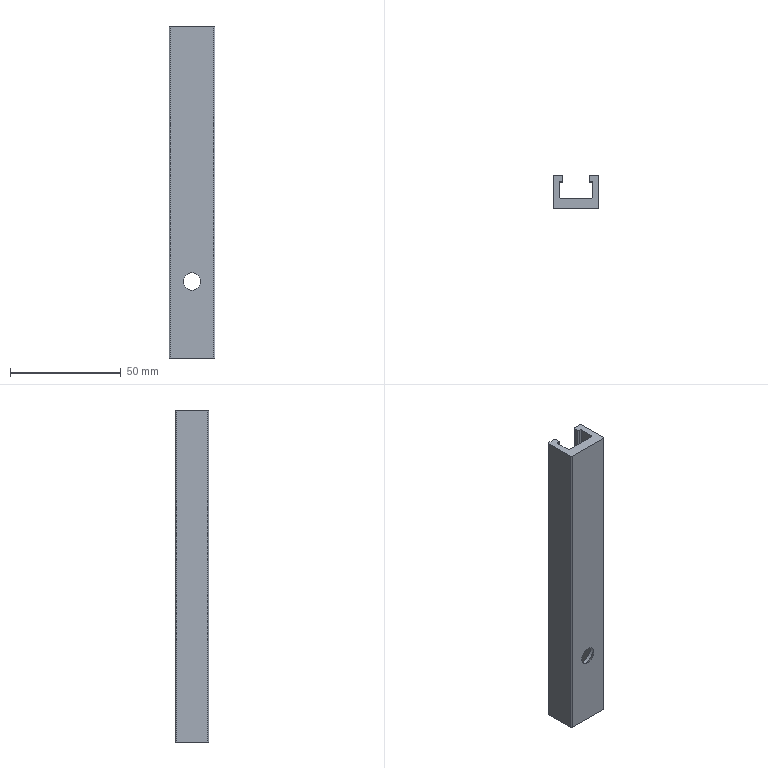Part | SolidWorks | features BaseBody 1 | 1 solid | 30 faces | box 20.769 x 15 x 150 mm | volume 24119 mm3 | cylinder 14 | plane 14 | cone 2 | commonest cylinder face diameters 0.923 x10 1.846 x2 13.846 x2
STEP:
#1=CARTESIAN_POINT('',(-21.677,381.039,171.154));
#2=VERTEX_POINT('',#1);
#3=CARTESIAN_POINT('',(-13.83,381.039,171.154));
#4=VERTEX_POINT('',#3);
#5=CARTESIAN_POINT('',(-17.753,381.039,171.154));
#6=DIRECTION('',(0.,-1.,0.));
#7=DIRECTION('',(-1.,0.,0.));
#8=AXIS2_PLACEMENT_3D('',#5,#6,#7);
#9=CIRCLE('',#8,3.923);
#10=EDGE_CURVE('',#2,#4,#9,.T.);
#11=ORIENTED_EDGE('',*,*,#10,.T.);
#12=CARTESIAN_POINT('',(-10.83,384.039,171.154));
#13=VERTEX_POINT('',#12);
#14=CARTESIAN_POINT('',(-10.83,384.039,171.154));
#15=DIRECTION('',(0.7071,0.7071,0.));
#16=VECTOR('',#15,1000.);
#17=LINE('',#14,#16);
#18=EDGE_CURVE('',#4,#13,#17,.T.);
#19=ORIENTED_EDGE('',*,*,#18,.T.);
#20=CARTESIAN_POINT('',(-17.753,384.039,164.231));
#21=VERTEX_POINT('',#20);
#22=CARTESIAN_POINT('',(-17.753,384.039,171.154));
#23=DIRECTION('',(0.,-1.,0.));
#24=DIRECTION('',(0.,0.,1.));
#25=AXIS2_PLACEMENT_3D('',#22,#23,#24);
#26=CIRCLE('',#25,6.923);
#27=EDGE_CURVE('',#21,#13,#26,.T.);
#28=ORIENTED_EDGE('',*,*,#27,.F.);
#29=CARTESIAN_POINT('',(-24.677,384.039,171.154));
#30=VERTEX_POINT('',#29);
#31=CARTESIAN_POINT('',(-17.753,384.039,171.154));
#32=DIRECTION('',(0.,-1.,0.));
#33=DIRECTION('',(0.,0.,1.));
#34=AXIS2_PLACEMENT_3D('',#31,#32,#33);
#35=CIRCLE('',#34,6.923);
#36=EDGE_CURVE('',#30,#21,#35,.T.);
#37=ORIENTED_EDGE('',*,*,#36,.F.);
#38=CARTESIAN_POINT('',(-24.677,384.039,171.154));
#39=DIRECTION('',(-0.7071,0.7071,0.));
#40=VECTOR('',#39,1000.);
#41=LINE('',#38,#40);
#42=EDGE_CURVE('',#2,#30,#41,.T.);
#43=ORIENTED_EDGE('',*,*,#42,.F.);
#44=EDGE_LOOP('',(#11,#19,#28,#37,#43));
#45=FACE_OUTER_BOUND('',#44,.T.);
#46=CARTESIAN_POINT('',(-17.753,384.039,171.154));
#47=DIRECTION('',(0.,1.,0.));
#48=DIRECTION('',(-1.,0.,0.));
#49=AXIS2_PLACEMENT_3D('',#46,#47,#48);
#50=CONICAL_SURFACE('',#49,6.923,0.7854);
#51=ADVANCED_FACE('',(#45),#50,.F.);
#52=CARTESIAN_POINT('',(-17.753,384.039,178.077));
#53=VERTEX_POINT('',#52);
#54=CARTESIAN_POINT('',(-17.753,384.039,171.154));
#55=DIRECTION('',(0.,-1.,0.));
#56=DIRECTION('',(0.,0.,1.));
#57=AXIS2_PLACEMENT_3D('',#54,#55,#56);
#58=CIRCLE('',#57,6.923);
#59=EDGE_CURVE('',#53,#30,#58,.T.);
#60=ORIENTED_EDGE('',*,*,#59,.T.);
#61=ORIENTED_EDGE('',*,*,#36,.T.);
#62=CARTESIAN_POINT('',(-17.753,385.654,164.231));
#63=VERTEX_POINT('',#62);
#64=CARTESIAN_POINT('',(-17.753,381.039,164.231));
#65=DIRECTION('',(0.,1.,0.));
#66=VECTOR('',#65,1000.);
#67=LINE('',#64,#66);
#68=EDGE_CURVE('',#21,#63,#67,.T.);
#69=ORIENTED_EDGE('',*,*,#68,.T.);
#70=CARTESIAN_POINT('',(-17.753,385.654,178.077));
#71=VERTEX_POINT('',#70);
#72=CARTESIAN_POINT('',(-17.753,385.654,171.154));
#73=DIRECTION('',(0.,-1.,0.));
#74=DIRECTION('',(0.,0.,1.));
#75=AXIS2_PLACEMENT_3D('',#72,#73,#74);
#76=CIRCLE('',#75,6.923);
#77=EDGE_CURVE('',#71,#63,#76,.T.);
#78=ORIENTED_EDGE('',*,*,#77,.F.);
#79=CARTESIAN_POINT('',(-17.753,381.039,178.077));
#80=DIRECTION('',(0.,1.,0.));
#81=VECTOR('',#80,1000.);
#82=LINE('',#79,#81);
#83=EDGE_CURVE('',#53,#71,#82,.T.);
#84=ORIENTED_EDGE('',*,*,#83,.F.);
#85=EDGE_LOOP('',(#60,#61,#69,#78,#84));
#86=FACE_OUTER_BOUND('',#85,.T.);
#87=CARTESIAN_POINT('',(-17.753,381.039,171.154));
#88=DIRECTION('',(0.,1.,0.));
#89=DIRECTION('',(0.,0.,1.));
#90=AXIS2_PLACEMENT_3D('',#87,#88,#89);
#91=CYLINDRICAL_SURFACE('',#90,6.923);
#92=ADVANCED_FACE('',(#86),#91,.F.);
#93=ORIENTED_EDGE('',*,*,#10,.F.);
#94=CARTESIAN_POINT('',(-17.753,381.039,171.154));
#95=DIRECTION('',(0.,-1.,0.));
#96=DIRECTION('',(-1.,0.,0.));
#97=AXIS2_PLACEMENT_3D('',#94,#95,#96);
#98=CIRCLE('',#97,3.923);
#99=EDGE_CURVE('',#4,#2,#98,.T.);
#100=ORIENTED_EDGE('',*,*,#99,.F.);
#101=EDGE_LOOP('',(#93,#100));
#102=FACE_BOUND('',#101,.T.);
#103=CARTESIAN_POINT('',(-7.83,381.039,286.538));
#104=VERTEX_POINT('',#103);
#105=CARTESIAN_POINT('',(-7.83,381.039,136.538));
#106=VERTEX_POINT('',#105);
#107=CARTESIAN_POINT('',(-7.83,381.039,136.538));
#108=DIRECTION('',(0.,0.,-1.));
#109=VECTOR('',#108,1000.);
#110=LINE('',#107,#109);
#111=EDGE_CURVE('',#104,#106,#110,.T.);
#112=ORIENTED_EDGE('',*,*,#111,.F.);
#113=CARTESIAN_POINT('',(-27.677,381.039,286.538));
#114=VERTEX_POINT('',#113);
#115=CARTESIAN_POINT('',(-7.83,381.039,286.538));
#116=DIRECTION('',(1.,0.,0.));
#117=VECTOR('',#116,1000.);
#118=LINE('',#115,#117);
#119=EDGE_CURVE('',#114,#104,#118,.T.);
#120=ORIENTED_EDGE('',*,*,#119,.F.);
#121=CARTESIAN_POINT('',(-27.677,381.039,136.538));
#122=VERTEX_POINT('',#121);
#123=CARTESIAN_POINT('',(-27.677,381.039,136.538));
#124=DIRECTION('',(0.,0.,1.));
#125=VECTOR('',#124,1000.);
#126=LINE('',#123,#125);
#127=EDGE_CURVE('',#122,#114,#126,.T.);
#128=ORIENTED_EDGE('',*,*,#127,.F.);
#129=CARTESIAN_POINT('',(-7.83,381.039,136.538));
#130=DIRECTION('',(-1.,0.,0.));
#131=VECTOR('',#130,1000.);
#132=LINE('',#129,#131);
#133=EDGE_CURVE('',#106,#122,#132,.T.);
#134=ORIENTED_EDGE('',*,*,#133,.F.);
#135=EDGE_LOOP('',(#112,#120,#128,#134));
#136=FACE_OUTER_BOUND('',#135,.T.);
#137=CARTESIAN_POINT('',(-7.83,381.039,136.538));
#138=DIRECTION('',(0.,1.,0.));
#139=DIRECTION('',(0.,0.,1.));
#140=AXIS2_PLACEMENT_3D('',#137,#138,#139);
#141=PLANE('',#140);
#142=ADVANCED_FACE('',(#102,#136),#141,.F.);
#143=ORIENTED_EDGE('',*,*,#18,.F.);
#144=ORIENTED_EDGE('',*,*,#99,.T.);
#145=ORIENTED_EDGE('',*,*,#42,.T.);
#146=ORIENTED_EDGE('',*,*,#59,.F.);
#147=CARTESIAN_POINT('',(-17.753,384.039,171.154));
#148=DIRECTION('',(0.,-1.,0.));
#149=DIRECTION('',(0.,0.,1.));
#150=AXIS2_PLACEMENT_3D('',#147,#148,#149);
#151=CIRCLE('',#150,6.923);
#152=EDGE_CURVE('',#13,#53,#151,.T.);
#153=ORIENTED_EDGE('',*,*,#152,.F.);
#154=EDGE_LOOP('',(#143,#144,#145,#146,#153));
#155=FACE_OUTER_BOUND('',#154,.T.);
#156=CARTESIAN_POINT('',(-17.753,384.039,171.154));
#157=DIRECTION('',(0.,1.,0.));
#158=DIRECTION('',(-1.,0.,0.));
#159=AXIS2_PLACEMENT_3D('',#156,#157,#158);
#160=CONICAL_SURFACE('',#159,6.923,0.7854);
#161=ADVANCED_FACE('',(#155),#160,.F.);
#162=CARTESIAN_POINT('',(-11.753,395.115,136.538));
#163=VERTEX_POINT('',#162);
#164=CARTESIAN_POINT('',(-10.83,396.039,136.538));
#165=VERTEX_POINT('',#164);
#166=CARTESIAN_POINT('',(-10.83,395.115,136.538));
#167=DIRECTION('',(0.,0.,-1.));
#168=DIRECTION('',(-1.,0.,0.));
#169=AXIS2_PLACEMENT_3D('',#166,#167,#168);
#170=CIRCLE('',#169,0.9231);
#171=EDGE_CURVE('',#163,#165,#170,.T.);
#172=ORIENTED_EDGE('',*,*,#171,.T.);
#173=CARTESIAN_POINT('',(-7.83,396.039,136.538));
#174=VERTEX_POINT('',#173);
#175=CARTESIAN_POINT('',(-7.83,396.039,136.538));
#176=DIRECTION('',(1.,0.,0.));
#177=VECTOR('',#176,1000.);
#178=LINE('',#175,#177);
#179=EDGE_CURVE('',#165,#174,#178,.T.);
#180=ORIENTED_EDGE('',*,*,#179,.T.);
#181=CARTESIAN_POINT('',(-7.369,395.577,136.538));
#182=VERTEX_POINT('',#181);
#183=CARTESIAN_POINT('',(-7.83,395.577,136.538));
#184=DIRECTION('',(0.,0.,-1.));
#185=DIRECTION('',(-1.,0.,0.));
#186=AXIS2_PLACEMENT_3D('',#183,#184,#185);
#187=CIRCLE('',#186,0.4615);
#188=EDGE_CURVE('',#174,#182,#187,.T.);
#189=ORIENTED_EDGE('',*,*,#188,.T.);
#190=CARTESIAN_POINT('',(-7.369,381.5,136.538));
#191=VERTEX_POINT('',#190);
#192=CARTESIAN_POINT('',(-7.369,381.5,136.538));
#193=DIRECTION('',(0.,-1.,0.));
#194=VECTOR('',#193,1000.);
#195=LINE('',#192,#194);
#196=EDGE_CURVE('',#182,#191,#195,.T.);
#197=ORIENTED_EDGE('',*,*,#196,.T.);
#198=CARTESIAN_POINT('',(-7.83,381.5,136.538));
#199=DIRECTION('',(0.,0.,-1.));
#200=DIRECTION('',(-1.,0.,0.));
#201=AXIS2_PLACEMENT_3D('',#198,#199,#200);
#202=CIRCLE('',#201,0.4615);
#203=EDGE_CURVE('',#191,#106,#202,.T.);
#204=ORIENTED_EDGE('',*,*,#203,.T.);
#205=ORIENTED_EDGE('',*,*,#133,.T.);
#206=CARTESIAN_POINT('',(-28.138,381.5,136.538));
#207=VERTEX_POINT('',#206);
#208=CARTESIAN_POINT('',(-27.677,381.5,136.538));
#209=DIRECTION('',(0.,0.,-1.));
#210=DIRECTION('',(-1.,0.,0.));
#211=AXIS2_PLACEMENT_3D('',#208,#209,#210);
#212=CIRCLE('',#211,0.4615);
#213=EDGE_CURVE('',#122,#207,#212,.T.);
#214=ORIENTED_EDGE('',*,*,#213,.T.);
#215=CARTESIAN_POINT('',(-28.138,395.577,136.538));
#216=VERTEX_POINT('',#215);
#217=CARTESIAN_POINT('',(-28.138,381.5,136.538));
#218=DIRECTION('',(0.,1.,0.));
#219=VECTOR('',#218,1000.);
#220=LINE('',#217,#219);
#221=EDGE_CURVE('',#207,#216,#220,.T.);
#222=ORIENTED_EDGE('',*,*,#221,.T.);
#223=CARTESIAN_POINT('',(-27.677,396.039,136.538));
#224=VERTEX_POINT('',#223);
#225=CARTESIAN_POINT('',(-27.677,395.577,136.538));
#226=DIRECTION('',(0.,0.,-1.));
#227=DIRECTION('',(-1.,0.,0.));
#228=AXIS2_PLACEMENT_3D('',#225,#226,#227);
#229=CIRCLE('',#228,0.4615);
#230=EDGE_CURVE('',#216,#224,#229,.T.);
#231=ORIENTED_EDGE('',*,*,#230,.T.);
#232=CARTESIAN_POINT('',(-24.677,396.039,136.538));
#233=VERTEX_POINT('',#232);
#234=CARTESIAN_POINT('',(-7.83,396.039,136.538));
#235=DIRECTION('',(1.,0.,0.));
#236=VECTOR('',#235,1000.);
#237=LINE('',#234,#236);
#238=EDGE_CURVE('',#224,#233,#237,.T.);
#239=ORIENTED_EDGE('',*,*,#238,.T.);
#240=CARTESIAN_POINT('',(-23.753,395.115,136.538));
#241=VERTEX_POINT('',#240);
#242=CARTESIAN_POINT('',(-24.677,395.115,136.538));
#243=DIRECTION('',(0.,0.,-1.));
#244=DIRECTION('',(-1.,0.,0.));
#245=AXIS2_PLACEMENT_3D('',#242,#243,#244);
#246=CIRCLE('',#245,0.9231);
#247=EDGE_CURVE('',#233,#241,#246,.T.);
#248=ORIENTED_EDGE('',*,*,#247,.T.);
#249=CARTESIAN_POINT('',(-23.753,393.5,136.538));
#250=VERTEX_POINT('',#249);
#251=CARTESIAN_POINT('',(-23.753,381.5,136.538));
#252=DIRECTION('',(0.,-1.,0.));
#253=VECTOR('',#252,1000.);
#254=LINE('',#251,#253);
#255=EDGE_CURVE('',#241,#250,#254,.T.);
#256=ORIENTED_EDGE('',*,*,#255,.T.);
#257=CARTESIAN_POINT('',(-24.215,393.039,136.538));
#258=VERTEX_POINT('',#257);
#259=CARTESIAN_POINT('',(-24.215,393.5,136.538));
#260=DIRECTION('',(0.,0.,-1.));
#261=DIRECTION('',(-1.,0.,0.));
#262=AXIS2_PLACEMENT_3D('',#259,#260,#261);
#263=CIRCLE('',#262,0.4615);
#264=EDGE_CURVE('',#250,#258,#263,.T.);
#265=ORIENTED_EDGE('',*,*,#264,.T.);
#266=CARTESIAN_POINT('',(-24.792,393.039,136.538));
#267=VERTEX_POINT('',#266);
#268=CARTESIAN_POINT('',(-7.83,393.039,136.538));
#269=DIRECTION('',(-1.,0.,0.));
#270=VECTOR('',#269,1000.);
#271=LINE('',#268,#270);
#272=EDGE_CURVE('',#258,#267,#271,.T.);
#273=ORIENTED_EDGE('',*,*,#272,.T.);
#274=CARTESIAN_POINT('',(-25.253,392.577,136.538));
#275=VERTEX_POINT('',#274);
#276=CARTESIAN_POINT('',(-24.792,392.577,136.538));
#277=DIRECTION('',(0.,0.,1.));
#278=DIRECTION('',(-1.,0.,0.));
#279=AXIS2_PLACEMENT_3D('',#276,#277,#278);
#280=CIRCLE('',#279,0.4615);
#281=EDGE_CURVE('',#267,#275,#280,.T.);
#282=ORIENTED_EDGE('',*,*,#281,.T.);
#283=CARTESIAN_POINT('',(-25.253,386.115,136.538));
#284=VERTEX_POINT('',#283);
#285=CARTESIAN_POINT('',(-25.253,381.5,136.538));
#286=DIRECTION('',(0.,-1.,0.));
#287=VECTOR('',#286,1000.);
#288=LINE('',#285,#287);
#289=EDGE_CURVE('',#275,#284,#288,.T.);
#290=ORIENTED_EDGE('',*,*,#289,.T.);
#291=CARTESIAN_POINT('',(-24.792,385.654,136.538));
#292=VERTEX_POINT('',#291);
#293=CARTESIAN_POINT('',(-24.792,386.115,136.538));
#294=DIRECTION('',(0.,0.,1.));
#295=DIRECTION('',(-1.,0.,0.));
#296=AXIS2_PLACEMENT_3D('',#293,#294,#295);
#297=CIRCLE('',#296,0.4615);
#298=EDGE_CURVE('',#284,#292,#297,.T.);
#299=ORIENTED_EDGE('',*,*,#298,.T.);
#300=CARTESIAN_POINT('',(-10.715,385.654,136.538));
#301=VERTEX_POINT('',#300);
#302=CARTESIAN_POINT('',(-7.83,385.654,136.538));
#303=DIRECTION('',(1.,0.,0.));
#304=VECTOR('',#303,1000.);
#305=LINE('',#302,#304);
#306=EDGE_CURVE('',#292,#301,#305,.T.);
#307=ORIENTED_EDGE('',*,*,#306,.T.);
#308=CARTESIAN_POINT('',(-10.253,386.115,136.538));
#309=VERTEX_POINT('',#308);
#310=CARTESIAN_POINT('',(-10.715,386.115,136.538));
#311=DIRECTION('',(0.,0.,1.));
#312=DIRECTION('',(-1.,0.,0.));
#313=AXIS2_PLACEMENT_3D('',#310,#311,#312);
#314=CIRCLE('',#313,0.4615);
#315=EDGE_CURVE('',#301,#309,#314,.T.);
#316=ORIENTED_EDGE('',*,*,#315,.T.);
#317=CARTESIAN_POINT('',(-10.253,392.577,136.538));
#318=VERTEX_POINT('',#317);
#319=CARTESIAN_POINT('',(-10.253,381.5,136.538));
#320=DIRECTION('',(0.,1.,0.));
#321=VECTOR('',#320,1000.);
#322=LINE('',#319,#321);
#323=EDGE_CURVE('',#309,#318,#322,.T.);
#324=ORIENTED_EDGE('',*,*,#323,.T.);
#325=CARTESIAN_POINT('',(-10.715,393.039,136.538));
#326=VERTEX_POINT('',#325);
#327=CARTESIAN_POINT('',(-10.715,392.577,136.538));
#328=DIRECTION('',(0.,0.,1.));
#329=DIRECTION('',(-1.,0.,0.));
#330=AXIS2_PLACEMENT_3D('',#327,#328,#329);
#331=CIRCLE('',#330,0.4615);
#332=EDGE_CURVE('',#318,#326,#331,.T.);
#333=ORIENTED_EDGE('',*,*,#332,.T.);
#334=CARTESIAN_POINT('',(-11.292,393.039,136.538));
#335=VERTEX_POINT('',#334);
#336=CARTESIAN_POINT('',(-7.83,393.039,136.538));
#337=DIRECTION('',(-1.,0.,0.));
#338=VECTOR('',#337,1000.);
#339=LINE('',#336,#338);
#340=EDGE_CURVE('',#326,#335,#339,.T.);
#341=ORIENTED_EDGE('',*,*,#340,.T.);
#342=CARTESIAN_POINT('',(-11.753,393.5,136.538));
#343=VERTEX_POINT('',#342);
#344=CARTESIAN_POINT('',(-11.292,393.5,136.538));
#345=DIRECTION('',(0.,0.,-1.));
#346=DIRECTION('',(-1.,0.,0.));
#347=AXIS2_PLACEMENT_3D('',#344,#345,#346);
#348=CIRCLE('',#347,0.4615);
#349=EDGE_CURVE('',#335,#343,#348,.T.);
#350=ORIENTED_EDGE('',*,*,#349,.T.);
#351=CARTESIAN_POINT('',(-11.753,381.5,136.538));
#352=DIRECTION('',(0.,1.,0.));
#353=VECTOR('',#352,1000.);
#354=LINE('',#351,#353);
#355=EDGE_CURVE('',#343,#163,#354,.T.);
#356=ORIENTED_EDGE('',*,*,#355,.T.);
#357=EDGE_LOOP('',(#172,#180,#189,#197,#204,#205,#214,#222,#231,#239,#248,#256,#265,#273,#282,#290,#299,#307,#316,#324,#333,#341,#350,#356));
#358=FACE_OUTER_BOUND('',#357,.T.);
#359=CARTESIAN_POINT('',(-7.83,381.5,136.538));
#360=DIRECTION('',(0.,0.,-1.));
#361=DIRECTION('',(-1.,0.,0.));
#362=AXIS2_PLACEMENT_3D('',#359,#360,#361);
#363=PLANE('',#362);
#364=ADVANCED_FACE('',(#358),#363,.T.);
#365=ORIENTED_EDGE('',*,*,#111,.T.);
#366=ORIENTED_EDGE('',*,*,#203,.F.);
#367=CARTESIAN_POINT('',(-7.369,381.5,286.538));
#368=VERTEX_POINT('',#367);
#369=CARTESIAN_POINT('',(-7.369,381.5,136.538));
#370=DIRECTION('',(0.,0.,1.));
#371=VECTOR('',#370,1000.);
#372=LINE('',#369,#371);
#373=EDGE_CURVE('',#191,#368,#372,.T.);
#374=ORIENTED_EDGE('',*,*,#373,.T.);
#375=CARTESIAN_POINT('',(-7.83,381.5,286.538));
#376=DIRECTION('',(0.,0.,-1.));
#377=DIRECTION('',(-1.,0.,0.));
#378=AXIS2_PLACEMENT_3D('',#375,#376,#377);
#379=CIRCLE('',#378,0.4615);
#380=EDGE_CURVE('',#368,#104,#379,.T.);
#381=ORIENTED_EDGE('',*,*,#380,.T.);
#382=EDGE_LOOP('',(#365,#366,#374,#381));
#383=FACE_OUTER_BOUND('',#382,.T.);
#384=CARTESIAN_POINT('',(-7.83,381.5,136.538));
#385=DIRECTION('',(0.,0.,-1.));
#386=DIRECTION('',(-1.,0.,0.));
#387=AXIS2_PLACEMENT_3D('',#384,#385,#386);
#388=CYLINDRICAL_SURFACE('',#387,0.4615);
#389=ADVANCED_FACE('',(#383),#388,.T.);
#390=CARTESIAN_POINT('',(-11.753,395.115,286.538));
#391=VERTEX_POINT('',#390);
#392=CARTESIAN_POINT('',(-10.83,396.039,286.538));
#393=VERTEX_POINT('',#392);
#394=CARTESIAN_POINT('',(-10.83,395.115,286.538));
#395=DIRECTION('',(0.,0.,-1.));
#396=DIRECTION('',(-1.,0.,0.));
#397=AXIS2_PLACEMENT_3D('',#394,#395,#396);
#398=CIRCLE('',#397,0.9231);
#399=EDGE_CURVE('',#391,#393,#398,.T.);
#400=ORIENTED_EDGE('',*,*,#399,.F.);
#401=CARTESIAN_POINT('',(-11.753,393.5,286.538));
#402=VERTEX_POINT('',#401);
#403=CARTESIAN_POINT('',(-11.753,381.5,286.538));
#404=DIRECTION('',(0.,1.,0.));
#405=VECTOR('',#404,1000.);
#406=LINE('',#403,#405);
#407=EDGE_CURVE('',#402,#391,#406,.T.);
#408=ORIENTED_EDGE('',*,*,#407,.F.);
#409=CARTESIAN_POINT('',(-11.292,393.039,286.538));
#410=VERTEX_POINT('',#409);
#411=CARTESIAN_POINT('',(-11.292,393.5,286.538));
#412=DIRECTION('',(0.,0.,-1.));
#413=DIRECTION('',(-1.,0.,0.));
#414=AXIS2_PLACEMENT_3D('',#411,#412,#413);
#415=CIRCLE('',#414,0.4615);
#416=EDGE_CURVE('',#410,#402,#415,.T.);
#417=ORIENTED_EDGE('',*,*,#416,.F.);
#418=CARTESIAN_POINT('',(-10.715,393.039,286.538));
#419=VERTEX_POINT('',#418);
#420=CARTESIAN_POINT('',(-7.83,393.039,286.538));
#421=DIRECTION('',(-1.,0.,0.));
#422=VECTOR('',#421,1000.);
#423=LINE('',#420,#422);
#424=EDGE_CURVE('',#419,#410,#423,.T.);
#425=ORIENTED_EDGE('',*,*,#424,.F.);
#426=CARTESIAN_POINT('',(-10.253,392.577,286.538));
#427=VERTEX_POINT('',#426);
#428=CARTESIAN_POINT('',(-10.715,392.577,286.538));
#429=DIRECTION('',(0.,0.,1.));
#430=DIRECTION('',(-1.,0.,0.));
#431=AXIS2_PLACEMENT_3D('',#428,#429,#430);
#432=CIRCLE('',#431,0.4615);
#433=EDGE_CURVE('',#427,#419,#432,.T.);
#434=ORIENTED_EDGE('',*,*,#433,.F.);
#435=CARTESIAN_POINT('',(-10.253,386.115,286.538));
#436=VERTEX_POINT('',#435);
#437=CARTESIAN_POINT('',(-10.253,381.5,286.538));
#438=DIRECTION('',(0.,1.,0.));
#439=VECTOR('',#438,1000.);
#440=LINE('',#437,#439);
#441=EDGE_CURVE('',#436,#427,#440,.T.);
#442=ORIENTED_EDGE('',*,*,#441,.F.);
#443=CARTESIAN_POINT('',(-10.715,385.654,286.538));
#444=VERTEX_POINT('',#443);
#445=CARTESIAN_POINT('',(-10.715,386.115,286.538));
#446=DIRECTION('',(0.,0.,1.));
#447=DIRECTION('',(-1.,0.,0.));
#448=AXIS2_PLACEMENT_3D('',#445,#446,#447);
#449=CIRCLE('',#448,0.4615);
#450=EDGE_CURVE('',#444,#436,#449,.T.);
#451=ORIENTED_EDGE('',*,*,#450,.F.);
#452=CARTESIAN_POINT('',(-24.792,385.654,286.538));
#453=VERTEX_POINT('',#452);
#454=CARTESIAN_POINT('',(-7.83,385.654,286.538));
#455=DIRECTION('',(1.,0.,0.));
#456=VECTOR('',#455,1000.);
#457=LINE('',#454,#456);
#458=EDGE_CURVE('',#453,#444,#457,.T.);
#459=ORIENTED_EDGE('',*,*,#458,.F.);
#460=CARTESIAN_POINT('',(-25.253,386.115,286.538));
#461=VERTEX_POINT('',#460);
#462=CARTESIAN_POINT('',(-24.792,386.115,286.538));
#463=DIRECTION('',(0.,0.,1.));
#464=DIRECTION('',(-1.,0.,0.));
#465=AXIS2_PLACEMENT_3D('',#462,#463,#464);
#466=CIRCLE('',#465,0.4615);
#467=EDGE_CURVE('',#461,#453,#466,.T.);
#468=ORIENTED_EDGE('',*,*,#467,.F.);
#469=CARTESIAN_POINT('',(-25.253,392.577,286.538));
#470=VERTEX_POINT('',#469);
#471=CARTESIAN_POINT('',(-25.253,381.5,286.538));
#472=DIRECTION('',(0.,-1.,0.));
#473=VECTOR('',#472,1000.);
#474=LINE('',#471,#473);
#475=EDGE_CURVE('',#470,#461,#474,.T.);
#476=ORIENTED_EDGE('',*,*,#475,.F.);
#477=CARTESIAN_POINT('',(-24.792,393.039,286.538));
#478=VERTEX_POINT('',#477);
#479=CARTESIAN_POINT('',(-24.792,392.577,286.538));
#480=DIRECTION('',(0.,0.,1.));
#481=DIRECTION('',(-1.,0.,0.));
#482=AXIS2_PLACEMENT_3D('',#479,#480,#481);
#483=CIRCLE('',#482,0.4615);
#484=EDGE_CURVE('',#478,#470,#483,.T.);
#485=ORIENTED_EDGE('',*,*,#484,.F.);
#486=CARTESIAN_POINT('',(-24.215,393.039,286.538));
#487=VERTEX_POINT('',#486);
#488=CARTESIAN_POINT('',(-7.83,393.039,286.538));
#489=DIRECTION('',(-1.,0.,0.));
#490=VECTOR('',#489,1000.);
#491=LINE('',#488,#490);
#492=EDGE_CURVE('',#487,#478,#491,.T.);
#493=ORIENTED_EDGE('',*,*,#492,.F.);
#494=CARTESIAN_POINT('',(-23.753,393.5,286.538));
#495=VERTEX_POINT('',#494);
#496=CARTESIAN_POINT('',(-24.215,393.5,286.538));
#497=DIRECTION('',(0.,0.,-1.));
#498=DIRECTION('',(-1.,0.,0.));
#499=AXIS2_PLACEMENT_3D('',#496,#497,#498);
#500=CIRCLE('',#499,0.4615);
#501=EDGE_CURVE('',#495,#487,#500,.T.);
#502=ORIENTED_EDGE('',*,*,#501,.F.);
#503=CARTESIAN_POINT('',(-23.753,395.115,286.538));
#504=VERTEX_POINT('',#503);
#505=CARTESIAN_POINT('',(-23.753,381.5,286.538));
#506=DIRECTION('',(0.,-1.,0.));
#507=VECTOR('',#506,1000.);
#508=LINE('',#505,#507);
#509=EDGE_CURVE('',#504,#495,#508,.T.);
#510=ORIENTED_EDGE('',*,*,#509,.F.);
#511=CARTESIAN_POINT('',(-24.677,396.039,286.538));
#512=VERTEX_POINT('',#511);
#513=CARTESIAN_POINT('',(-24.677,395.115,286.538));
#514=DIRECTION('',(0.,0.,-1.));
#515=DIRECTION('',(-1.,0.,0.));
#516=AXIS2_PLACEMENT_3D('',#513,#514,#515);
#517=CIRCLE('',#516,0.9231);
#518=EDGE_CURVE('',#512,#504,#517,.T.);
#519=ORIENTED_EDGE('',*,*,#518,.F.);
#520=CARTESIAN_POINT('',(-27.677,396.039,286.538));
#521=VERTEX_POINT('',#520);
#522=CARTESIAN_POINT('',(-7.83,396.039,286.538));
#523=DIRECTION('',(1.,0.,0.));
#524=VECTOR('',#523,1000.);
#525=LINE('',#522,#524);
#526=EDGE_CURVE('',#521,#512,#525,.T.);
#527=ORIENTED_EDGE('',*,*,#526,.F.);
#528=CARTESIAN_POINT('',(-28.138,395.577,286.538));
#529=VERTEX_POINT('',#528);
#530=CARTESIAN_POINT('',(-27.677,395.577,286.538));
#531=DIRECTION('',(0.,0.,-1.));
#532=DIRECTION('',(-1.,0.,0.));
#533=AXIS2_PLACEMENT_3D('',#530,#531,#532);
#534=CIRCLE('',#533,0.4615);
#535=EDGE_CURVE('',#529,#521,#534,.T.);
#536=ORIENTED_EDGE('',*,*,#535,.F.);
#537=CARTESIAN_POINT('',(-28.138,381.5,286.538));
#538=VERTEX_POINT('',#537);
#539=CARTESIAN_POINT('',(-28.138,381.5,286.538));
#540=DIRECTION('',(0.,1.,0.));
#541=VECTOR('',#540,1000.);
#542=LINE('',#539,#541);
#543=EDGE_CURVE('',#538,#529,#542,.T.);
#544=ORIENTED_EDGE('',*,*,#543,.F.);
#545=CARTESIAN_POINT('',(-27.677,381.5,286.538));
#546=DIRECTION('',(0.,0.,-1.));
#547=DIRECTION('',(-1.,0.,0.));
#548=AXIS2_PLACEMENT_3D('',#545,#546,#547);
#549=CIRCLE('',#548,0.4615);
#550=EDGE_CURVE('',#114,#538,#549,.T.);
#551=ORIENTED_EDGE('',*,*,#550,.F.);
#552=ORIENTED_EDGE('',*,*,#119,.T.);
#553=ORIENTED_EDGE('',*,*,#380,.F.);
#554=CARTESIAN_POINT('',(-7.369,395.577,286.538));
#555=VERTEX_POINT('',#554);
#556=CARTESIAN_POINT('',(-7.369,381.5,286.538));
#557=DIRECTION('',(0.,-1.,0.));
#558=VECTOR('',#557,1000.);
#559=LINE('',#556,#558);
#560=EDGE_CURVE('',#555,#368,#559,.T.);
#561=ORIENTED_EDGE('',*,*,#560,.F.);
#562=CARTESIAN_POINT('',(-7.83,396.039,286.538));
#563=VERTEX_POINT('',#562);
#564=CARTESIAN_POINT('',(-7.83,395.577,286.538));
#565=DIRECTION('',(0.,0.,-1.));
#566=DIRECTION('',(-1.,0.,0.));
#567=AXIS2_PLACEMENT_3D('',#564,#565,#566);
#568=CIRCLE('',#567,0.4615);
#569=EDGE_CURVE('',#563,#555,#568,.T.);
#570=ORIENTED_EDGE('',*,*,#569,.F.);
#571=CARTESIAN_POINT('',(-7.83,396.039,286.538));
#572=DIRECTION('',(1.,0.,0.));
#573=VECTOR('',#572,1000.);
#574=LINE('',#571,#573);
#575=EDGE_CURVE('',#393,#563,#574,.T.);
#576=ORIENTED_EDGE('',*,*,#575,.F.);
#577=EDGE_LOOP('',(#400,#408,#417,#425,#434,#442,#451,#459,#468,#476,#485,#493,#502,#510,#519,#527,#536,#544,#551,#552,#553,#561,#570,#576));
#578=FACE_OUTER_BOUND('',#577,.T.);
#579=CARTESIAN_POINT('',(-7.83,381.5,286.538));
#580=DIRECTION('',(0.,0.,-1.));
#581=DIRECTION('',(-1.,0.,0.));
#582=AXIS2_PLACEMENT_3D('',#579,#580,#581);
#583=PLANE('',#582);
#584=ADVANCED_FACE('',(#578),#583,.F.);
#585=CARTESIAN_POINT('',(-28.138,381.5,136.538));
#586=DIRECTION('',(0.,0.,-1.));
#587=VECTOR('',#586,1000.);
#588=LINE('',#585,#587);
#589=EDGE_CURVE('',#538,#207,#588,.T.);
#590=ORIENTED_EDGE('',*,*,#589,.T.);
#591=ORIENTED_EDGE('',*,*,#213,.F.);
#592=ORIENTED_EDGE('',*,*,#127,.T.);
#593=ORIENTED_EDGE('',*,*,#550,.T.);
#594=EDGE_LOOP('',(#590,#591,#592,#593));
#595=FACE_OUTER_BOUND('',#594,.T.);
#596=CARTESIAN_POINT('',(-27.677,381.5,136.538));
#597=DIRECTION('',(0.,0.,-1.));
#598=DIRECTION('',(-1.,0.,0.));
#599=AXIS2_PLACEMENT_3D('',#596,#597,#598);
#600=CYLINDRICAL_SURFACE('',#599,0.4615);
#601=ADVANCED_FACE('',(#595),#600,.T.);
#602=ORIENTED_EDGE('',*,*,#68,.F.);
#603=ORIENTED_EDGE('',*,*,#27,.T.);
#604=ORIENTED_EDGE('',*,*,#152,.T.);
#605=ORIENTED_EDGE('',*,*,#83,.T.);
#606=CARTESIAN_POINT('',(-17.753,385.654,171.154));
#607=DIRECTION('',(0.,-1.,0.));
#608=DIRECTION('',(0.,0.,1.));
#609=AXIS2_PLACEMENT_3D('',#606,#607,#608);
#610=CIRCLE('',#609,6.923);
#611=EDGE_CURVE('',#63,#71,#610,.T.);
#612=ORIENTED_EDGE('',*,*,#611,.F.);
#613=EDGE_LOOP('',(#602,#603,#604,#605,#612));
#614=FACE_OUTER_BOUND('',#613,.T.);
#615=CARTESIAN_POINT('',(-17.753,381.039,171.154));
#616=DIRECTION('',(0.,1.,0.));
#617=DIRECTION('',(0.,0.,1.));
#618=AXIS2_PLACEMENT_3D('',#615,#616,#617);
#619=CYLINDRICAL_SURFACE('',#618,6.923);
#620=ADVANCED_FACE('',(#614),#619,.F.);
#621=CARTESIAN_POINT('',(-10.83,396.039,136.538));
#622=DIRECTION('',(0.,0.,-1.));
#623=VECTOR('',#622,1000.);
#624=LINE('',#621,#623);
#625=EDGE_CURVE('',#393,#165,#624,.T.);
#626=ORIENTED_EDGE('',*,*,#625,.F.);
#627=ORIENTED_EDGE('',*,*,#575,.T.);
#628=CARTESIAN_POINT('',(-7.83,396.039,136.538));
#629=DIRECTION('',(0.,0.,1.));
#630=VECTOR('',#629,1000.);
#631=LINE('',#628,#630);
#632=EDGE_CURVE('',#174,#563,#631,.T.);
#633=ORIENTED_EDGE('',*,*,#632,.F.);
#634=ORIENTED_EDGE('',*,*,#179,.F.);
#635=EDGE_LOOP('',(#626,#627,#633,#634));
#636=FACE_OUTER_BOUND('',#635,.T.);
#637=CARTESIAN_POINT('',(-10.83,396.039,136.538));
#638=DIRECTION('',(0.,-1.,0.));
#639=DIRECTION('',(0.,0.,-1.));
#640=AXIS2_PLACEMENT_3D('',#637,#638,#639);
#641=PLANE('',#640);
#642=ADVANCED_FACE('',(#636),#641,.F.);
#643=ORIENTED_EDGE('',*,*,#625,.T.);
#644=ORIENTED_EDGE('',*,*,#171,.F.);
#645=CARTESIAN_POINT('',(-11.753,395.115,136.538));
#646=DIRECTION('',(0.,0.,1.));
#647=VECTOR('',#646,1000.);
#648=LINE('',#645,#647);
#649=EDGE_CURVE('',#163,#391,#648,.T.);
#650=ORIENTED_EDGE('',*,*,#649,.T.);
#651=ORIENTED_EDGE('',*,*,#399,.T.);
#652=EDGE_LOOP('',(#643,#644,#650,#651));
#653=FACE_OUTER_BOUND('',#652,.T.);
#654=CARTESIAN_POINT('',(-10.83,395.115,136.538));
#655=DIRECTION('',(0.,0.,-1.));
#656=DIRECTION('',(-1.,0.,0.));
#657=AXIS2_PLACEMENT_3D('',#654,#655,#656);
#658=CYLINDRICAL_SURFACE('',#657,0.9231);
#659=ADVANCED_FACE('',(#653),#658,.T.);
#660=CARTESIAN_POINT('',(-11.753,393.5,136.538));
#661=DIRECTION('',(0.,0.,-1.));
#662=VECTOR('',#661,1000.);
#663=LINE('',#660,#662);
#664=EDGE_CURVE('',#402,#343,#663,.T.);
#665=ORIENTED_EDGE('',*,*,#664,.F.);
#666=ORIENTED_EDGE('',*,*,#407,.T.);
#667=ORIENTED_EDGE('',*,*,#649,.F.);
#668=ORIENTED_EDGE('',*,*,#355,.F.);
#669=EDGE_LOOP('',(#665,#666,#667,#668));
#670=FACE_OUTER_BOUND('',#669,.T.);
#671=CARTESIAN_POINT('',(-11.753,393.5,136.538));
#672=DIRECTION('',(1.,0.,0.));
#673=DIRECTION('',(0.,0.,-1.));
#674=AXIS2_PLACEMENT_3D('',#671,#672,#673);
#675=PLANE('',#674);
#676=ADVANCED_FACE('',(#670),#675,.F.);
#677=ORIENTED_EDGE('',*,*,#664,.T.);
#678=ORIENTED_EDGE('',*,*,#349,.F.);
#679=CARTESIAN_POINT('',(-11.292,393.039,136.538));
#680=DIRECTION('',(0.,0.,1.));
#681=VECTOR('',#680,1000.);
#682=LINE('',#679,#681);
#683=EDGE_CURVE('',#335,#410,#682,.T.);
#684=ORIENTED_EDGE('',*,*,#683,.T.);
#685=ORIENTED_EDGE('',*,*,#416,.T.);
#686=EDGE_LOOP('',(#677,#678,#684,#685));
#687=FACE_OUTER_BOUND('',#686,.T.);
#688=CARTESIAN_POINT('',(-11.292,393.5,136.538));
#689=DIRECTION('',(0.,0.,-1.));
#690=DIRECTION('',(-1.,0.,0.));
#691=AXIS2_PLACEMENT_3D('',#688,#689,#690);
#692=CYLINDRICAL_SURFACE('',#691,0.4615);
#693=ADVANCED_FACE('',(#687),#692,.T.);
#694=CARTESIAN_POINT('',(-10.715,393.039,136.538));
#695=DIRECTION('',(0.,0.,-1.));
#696=VECTOR('',#695,1000.);
#697=LINE('',#694,#696);
#698=EDGE_CURVE('',#419,#326,#697,.T.);
#699=ORIENTED_EDGE('',*,*,#698,.F.);
#700=ORIENTED_EDGE('',*,*,#424,.T.);
#701=ORIENTED_EDGE('',*,*,#683,.F.);
#702=ORIENTED_EDGE('',*,*,#340,.F.);
#703=EDGE_LOOP('',(#699,#700,#701,#702));
#704=FACE_OUTER_BOUND('',#703,.T.);
#705=CARTESIAN_POINT('',(-10.715,393.039,136.538));
#706=DIRECTION('',(0.,1.,0.));
#707=DIRECTION('',(0.,0.,1.));
#708=AXIS2_PLACEMENT_3D('',#705,#706,#707);
#709=PLANE('',#708);
#710=ADVANCED_FACE('',(#704),#709,.F.);
#711=CARTESIAN_POINT('',(-10.253,392.577,136.538));
#712=DIRECTION('',(0.,0.,-1.));
#713=VECTOR('',#712,1000.);
#714=LINE('',#711,#713);
#715=EDGE_CURVE('',#427,#318,#714,.T.);
#716=ORIENTED_EDGE('',*,*,#715,.F.);
#717=ORIENTED_EDGE('',*,*,#433,.T.);
#718=ORIENTED_EDGE('',*,*,#698,.T.);
#719=ORIENTED_EDGE('',*,*,#332,.F.);
#720=EDGE_LOOP('',(#716,#717,#718,#719));
#721=FACE_OUTER_BOUND('',#720,.T.);
#722=CARTESIAN_POINT('',(-10.715,392.577,136.538));
#723=DIRECTION('',(0.,0.,-1.));
#724=DIRECTION('',(-1.,0.,0.));
#725=AXIS2_PLACEMENT_3D('',#722,#723,#724);
#726=CYLINDRICAL_SURFACE('',#725,0.4615);
#727=ADVANCED_FACE('',(#721),#726,.F.);
#728=CARTESIAN_POINT('',(-10.253,386.115,136.538));
#729=DIRECTION('',(0.,0.,-1.));
#730=VECTOR('',#729,1000.);
#731=LINE('',#728,#730);
#732=EDGE_CURVE('',#436,#309,#731,.T.);
#733=ORIENTED_EDGE('',*,*,#732,.F.);
#734=ORIENTED_EDGE('',*,*,#441,.T.);
#735=ORIENTED_EDGE('',*,*,#715,.T.);
#736=ORIENTED_EDGE('',*,*,#323,.F.);
#737=EDGE_LOOP('',(#733,#734,#735,#736));
#738=FACE_OUTER_BOUND('',#737,.T.);
#739=CARTESIAN_POINT('',(-10.253,386.115,136.538));
#740=DIRECTION('',(1.,0.,0.));
#741=DIRECTION('',(0.,0.,-1.));
#742=AXIS2_PLACEMENT_3D('',#739,#740,#741);
#743=PLANE('',#742);
#744=ADVANCED_FACE('',(#738),#743,.F.);
#745=CARTESIAN_POINT('',(-10.715,385.654,136.538));
#746=DIRECTION('',(0.,0.,-1.));
#747=VECTOR('',#746,1000.);
#748=LINE('',#745,#747);
#749=EDGE_CURVE('',#444,#301,#748,.T.);
#750=ORIENTED_EDGE('',*,*,#749,.F.);
#751=ORIENTED_EDGE('',*,*,#450,.T.);
#752=ORIENTED_EDGE('',*,*,#732,.T.);
#753=ORIENTED_EDGE('',*,*,#315,.F.);
#754=EDGE_LOOP('',(#750,#751,#752,#753));
#755=FACE_OUTER_BOUND('',#754,.T.);
#756=CARTESIAN_POINT('',(-10.715,386.115,136.538));
#757=DIRECTION('',(0.,0.,-1.));
#758=DIRECTION('',(-1.,0.,0.));
#759=AXIS2_PLACEMENT_3D('',#756,#757,#758);
#760=CYLINDRICAL_SURFACE('',#759,0.4615);
#761=ADVANCED_FACE('',(#755),#760,.F.);
#762=ORIENTED_EDGE('',*,*,#77,.T.);
#763=ORIENTED_EDGE('',*,*,#611,.T.);
#764=EDGE_LOOP('',(#762,#763));
#765=FACE_BOUND('',#764,.T.);
#766=CARTESIAN_POINT('',(-24.792,385.654,136.538));
#767=DIRECTION('',(0.,0.,-1.));
#768=VECTOR('',#767,1000.);
#769=LINE('',#766,#768);
#770=EDGE_CURVE('',#453,#292,#769,.T.);
#771=ORIENTED_EDGE('',*,*,#770,.F.);
#772=ORIENTED_EDGE('',*,*,#458,.T.);
#773=ORIENTED_EDGE('',*,*,#749,.T.);
#774=ORIENTED_EDGE('',*,*,#306,.F.);
#775=EDGE_LOOP('',(#771,#772,#773,#774));
#776=FACE_OUTER_BOUND('',#775,.T.);
#777=CARTESIAN_POINT('',(-24.792,385.654,136.538));
#778=DIRECTION('',(0.,-1.,0.));
#779=DIRECTION('',(0.,0.,-1.));
#780=AXIS2_PLACEMENT_3D('',#777,#778,#779);
#781=PLANE('',#780);
#782=ADVANCED_FACE('',(#765,#776),#781,.F.);
#783=CARTESIAN_POINT('',(-25.253,386.115,136.538));
#784=DIRECTION('',(0.,0.,-1.));
#785=VECTOR('',#784,1000.);
#786=LINE('',#783,#785);
#787=EDGE_CURVE('',#461,#284,#786,.T.);
#788=ORIENTED_EDGE('',*,*,#787,.F.);
#789=ORIENTED_EDGE('',*,*,#467,.T.);
#790=ORIENTED_EDGE('',*,*,#770,.T.);
#791=ORIENTED_EDGE('',*,*,#298,.F.);
#792=EDGE_LOOP('',(#788,#789,#790,#791));
#793=FACE_OUTER_BOUND('',#792,.T.);
#794=CARTESIAN_POINT('',(-24.792,386.115,136.538));
#795=DIRECTION('',(0.,0.,-1.));
#796=DIRECTION('',(-1.,0.,0.));
#797=AXIS2_PLACEMENT_3D('',#794,#795,#796);
#798=CYLINDRICAL_SURFACE('',#797,0.4615);
#799=ADVANCED_FACE('',(#793),#798,.F.);
#800=CARTESIAN_POINT('',(-25.253,392.577,136.538));
#801=DIRECTION('',(0.,0.,-1.));
#802=VECTOR('',#801,1000.);
#803=LINE('',#800,#802);
#804=EDGE_CURVE('',#470,#275,#803,.T.);
#805=ORIENTED_EDGE('',*,*,#804,.F.);
#806=ORIENTED_EDGE('',*,*,#475,.T.);
#807=ORIENTED_EDGE('',*,*,#787,.T.);
#808=ORIENTED_EDGE('',*,*,#289,.F.);
#809=EDGE_LOOP('',(#805,#806,#807,#808));
#810=FACE_OUTER_BOUND('',#809,.T.);
#811=CARTESIAN_POINT('',(-25.253,392.577,136.538));
#812=DIRECTION('',(-1.,0.,0.));
#813=DIRECTION('',(0.,0.,1.));
#814=AXIS2_PLACEMENT_3D('',#811,#812,#813);
#815=PLANE('',#814);
#816=ADVANCED_FACE('',(#810),#815,.F.);
#817=CARTESIAN_POINT('',(-24.792,393.039,136.538));
#818=DIRECTION('',(0.,0.,-1.));
#819=VECTOR('',#818,1000.);
#820=LINE('',#817,#819);
#821=EDGE_CURVE('',#478,#267,#820,.T.);
#822=ORIENTED_EDGE('',*,*,#821,.F.);
#823=ORIENTED_EDGE('',*,*,#484,.T.);
#824=ORIENTED_EDGE('',*,*,#804,.T.);
#825=ORIENTED_EDGE('',*,*,#281,.F.);
#826=EDGE_LOOP('',(#822,#823,#824,#825));
#827=FACE_OUTER_BOUND('',#826,.T.);
#828=CARTESIAN_POINT('',(-24.792,392.577,136.538));
#829=DIRECTION('',(0.,0.,-1.));
#830=DIRECTION('',(-1.,0.,0.));
#831=AXIS2_PLACEMENT_3D('',#828,#829,#830);
#832=CYLINDRICAL_SURFACE('',#831,0.4615);
#833=ADVANCED_FACE('',(#827),#832,.F.);
#834=CARTESIAN_POINT('',(-24.215,393.039,136.538));
#835=DIRECTION('',(0.,0.,-1.));
#836=VECTOR('',#835,1000.);
#837=LINE('',#834,#836);
#838=EDGE_CURVE('',#487,#258,#837,.T.);
#839=ORIENTED_EDGE('',*,*,#838,.F.);
#840=ORIENTED_EDGE('',*,*,#492,.T.);
#841=ORIENTED_EDGE('',*,*,#821,.T.);
#842=ORIENTED_EDGE('',*,*,#272,.F.);
#843=EDGE_LOOP('',(#839,#840,#841,#842));
#844=FACE_OUTER_BOUND('',#843,.T.);
#845=CARTESIAN_POINT('',(-24.215,393.039,136.538));
#846=DIRECTION('',(0.,1.,0.));
#847=DIRECTION('',(0.,0.,1.));
#848=AXIS2_PLACEMENT_3D('',#845,#846,#847);
#849=PLANE('',#848);
#850=ADVANCED_FACE('',(#844),#849,.F.);
#851=ORIENTED_EDGE('',*,*,#838,.T.);
#852=ORIENTED_EDGE('',*,*,#264,.F.);
#853=CARTESIAN_POINT('',(-23.753,393.5,136.538));
#854=DIRECTION('',(0.,0.,1.));
#855=VECTOR('',#854,1000.);
#856=LINE('',#853,#855);
#857=EDGE_CURVE('',#250,#495,#856,.T.);
#858=ORIENTED_EDGE('',*,*,#857,.T.);
#859=ORIENTED_EDGE('',*,*,#501,.T.);
#860=EDGE_LOOP('',(#851,#852,#858,#859));
#861=FACE_OUTER_BOUND('',#860,.T.);
#862=CARTESIAN_POINT('',(-24.215,393.5,136.538));
#863=DIRECTION('',(0.,0.,-1.));
#864=DIRECTION('',(-1.,0.,0.));
#865=AXIS2_PLACEMENT_3D('',#862,#863,#864);
#866=CYLINDRICAL_SURFACE('',#865,0.4615);
#867=ADVANCED_FACE('',(#861),#866,.T.);
#868=CARTESIAN_POINT('',(-23.753,395.115,136.538));
#869=DIRECTION('',(0.,0.,-1.));
#870=VECTOR('',#869,1000.);
#871=LINE('',#868,#870);
#872=EDGE_CURVE('',#504,#241,#871,.T.);
#873=ORIENTED_EDGE('',*,*,#872,.F.);
#874=ORIENTED_EDGE('',*,*,#509,.T.);
#875=ORIENTED_EDGE('',*,*,#857,.F.);
#876=ORIENTED_EDGE('',*,*,#255,.F.);
#877=EDGE_LOOP('',(#873,#874,#875,#876));
#878=FACE_OUTER_BOUND('',#877,.T.);
#879=CARTESIAN_POINT('',(-23.753,395.115,136.538));
#880=DIRECTION('',(-1.,0.,0.));
#881=DIRECTION('',(0.,0.,1.));
#882=AXIS2_PLACEMENT_3D('',#879,#880,#881);
#883=PLANE('',#882);
#884=ADVANCED_FACE('',(#878),#883,.F.);
#885=ORIENTED_EDGE('',*,*,#872,.T.);
#886=ORIENTED_EDGE('',*,*,#247,.F.);
#887=CARTESIAN_POINT('',(-24.677,396.039,136.538));
#888=DIRECTION('',(0.,0.,1.));
#889=VECTOR('',#888,1000.);
#890=LINE('',#887,#889);
#891=EDGE_CURVE('',#233,#512,#890,.T.);
#892=ORIENTED_EDGE('',*,*,#891,.T.);
#893=ORIENTED_EDGE('',*,*,#518,.T.);
#894=EDGE_LOOP('',(#885,#886,#892,#893));
#895=FACE_OUTER_BOUND('',#894,.T.);
#896=CARTESIAN_POINT('',(-24.677,395.115,136.538));
#897=DIRECTION('',(0.,0.,-1.));
#898=DIRECTION('',(-1.,0.,0.));
#899=AXIS2_PLACEMENT_3D('',#896,#897,#898);
#900=CYLINDRICAL_SURFACE('',#899,0.9231);
#901=ADVANCED_FACE('',(#895),#900,.T.);
#902=CARTESIAN_POINT('',(-27.677,396.039,136.538));
#903=DIRECTION('',(0.,0.,-1.));
#904=VECTOR('',#903,1000.);
#905=LINE('',#902,#904);
#906=EDGE_CURVE('',#521,#224,#905,.T.);
#907=ORIENTED_EDGE('',*,*,#906,.F.);
#908=ORIENTED_EDGE('',*,*,#526,.T.);
#909=ORIENTED_EDGE('',*,*,#891,.F.);
#910=ORIENTED_EDGE('',*,*,#238,.F.);
#911=EDGE_LOOP('',(#907,#908,#909,#910));
#912=FACE_OUTER_BOUND('',#911,.T.);
#913=CARTESIAN_POINT('',(-27.677,396.039,136.538));
#914=DIRECTION('',(0.,-1.,0.));
#915=DIRECTION('',(0.,0.,-1.));
#916=AXIS2_PLACEMENT_3D('',#913,#914,#915);
#917=PLANE('',#916);
#918=ADVANCED_FACE('',(#912),#917,.F.);
#919=ORIENTED_EDGE('',*,*,#906,.T.);
#920=ORIENTED_EDGE('',*,*,#230,.F.);
#921=CARTESIAN_POINT('',(-28.138,395.577,136.538));
#922=DIRECTION('',(0.,0.,1.));
#923=VECTOR('',#922,1000.);
#924=LINE('',#921,#923);
#925=EDGE_CURVE('',#216,#529,#924,.T.);
#926=ORIENTED_EDGE('',*,*,#925,.T.);
#927=ORIENTED_EDGE('',*,*,#535,.T.);
#928=EDGE_LOOP('',(#919,#920,#926,#927));
#929=FACE_OUTER_BOUND('',#928,.T.);
#930=CARTESIAN_POINT('',(-27.677,395.577,136.538));
#931=DIRECTION('',(0.,0.,-1.));
#932=DIRECTION('',(-1.,0.,0.));
#933=AXIS2_PLACEMENT_3D('',#930,#931,#932);
#934=CYLINDRICAL_SURFACE('',#933,0.4615);
#935=ADVANCED_FACE('',(#929),#934,.T.);
#936=ORIENTED_EDGE('',*,*,#589,.F.);
#937=ORIENTED_EDGE('',*,*,#543,.T.);
#938=ORIENTED_EDGE('',*,*,#925,.F.);
#939=ORIENTED_EDGE('',*,*,#221,.F.);
#940=EDGE_LOOP('',(#936,#937,#938,#939));
#941=FACE_OUTER_BOUND('',#940,.T.);
#942=CARTESIAN_POINT('',(-28.138,381.5,136.538));
#943=DIRECTION('',(1.,0.,0.));
#944=DIRECTION('',(0.,0.,-1.));
#945=AXIS2_PLACEMENT_3D('',#942,#943,#944);
#946=PLANE('',#945);
#947=ADVANCED_FACE('',(#941),#946,.F.);
#948=CARTESIAN_POINT('',(-7.369,395.577,136.538));
#949=DIRECTION('',(0.,0.,-1.));
#950=VECTOR('',#949,1000.);
#951=LINE('',#948,#950);
#952=EDGE_CURVE('',#555,#182,#951,.T.);
#953=ORIENTED_EDGE('',*,*,#952,.F.);
#954=ORIENTED_EDGE('',*,*,#560,.T.);
#955=ORIENTED_EDGE('',*,*,#373,.F.);
#956=ORIENTED_EDGE('',*,*,#196,.F.);
#957=EDGE_LOOP('',(#953,#954,#955,#956));
#958=FACE_OUTER_BOUND('',#957,.T.);
#959=CARTESIAN_POINT('',(-7.369,395.577,136.538));
#960=DIRECTION('',(-1.,0.,0.));
#961=DIRECTION('',(0.,0.,1.));
#962=AXIS2_PLACEMENT_3D('',#959,#960,#961);
#963=PLANE('',#962);
#964=ADVANCED_FACE('',(#958),#963,.F.);
#965=ORIENTED_EDGE('',*,*,#952,.T.);
#966=ORIENTED_EDGE('',*,*,#188,.F.);
#967=ORIENTED_EDGE('',*,*,#632,.T.);
#968=ORIENTED_EDGE('',*,*,#569,.T.);
#969=EDGE_LOOP('',(#965,#966,#967,#968));
#970=FACE_OUTER_BOUND('',#969,.T.);
#971=CARTESIAN_POINT('',(-7.83,395.577,136.538));
#972=DIRECTION('',(0.,0.,-1.));
#973=DIRECTION('',(-1.,0.,0.));
#974=AXIS2_PLACEMENT_3D('',#971,#972,#973);
#975=CYLINDRICAL_SURFACE('',#974,0.4615);
#976=ADVANCED_FACE('',(#970),#975,.T.);
#977=CLOSED_SHELL('',(#51,#92,#142,#161,#364,#389,#584,#601,#620,#642,#659,#676,#693,#710,#727,#744,#761,#782,#799,#816,#833,#850,#867,#884,#901,#918,#935,#947,#964,#976));
#978=MANIFOLD_SOLID_BREP('',#977);
#979=CARTESIAN_POINT('',(0.,0.,0.));
#980=DIRECTION('',(0.,0.,1.));
#981=DIRECTION('',(1.,0.,0.));
#982=AXIS2_PLACEMENT_3D('',#979,#980,#981);
#983=(LENGTH_UNIT()NAMED_UNIT(*)SI_UNIT(.MILLI.,.METRE.));
#984=UNCERTAINTY_MEASURE_WITH_UNIT(LENGTH_MEASURE(0.00001),#983,'','');
#985=(NAMED_UNIT(*)PLANE_ANGLE_UNIT()SI_UNIT($,.RADIAN.));
#986=(NAMED_UNIT(*)SI_UNIT($,.STERADIAN.)SOLID_ANGLE_UNIT());
#987=(GEOMETRIC_REPRESENTATION_CONTEXT(3)GLOBAL_UNCERTAINTY_ASSIGNED_CONTEXT((#984))GLOBAL_UNIT_ASSIGNED_CONTEXT((#983,#985,#986))REPRESENTATION_CONTEXT('',''));
#988=ADVANCED_BREP_SHAPE_REPRESENTATION('',(#978,#982),#987);